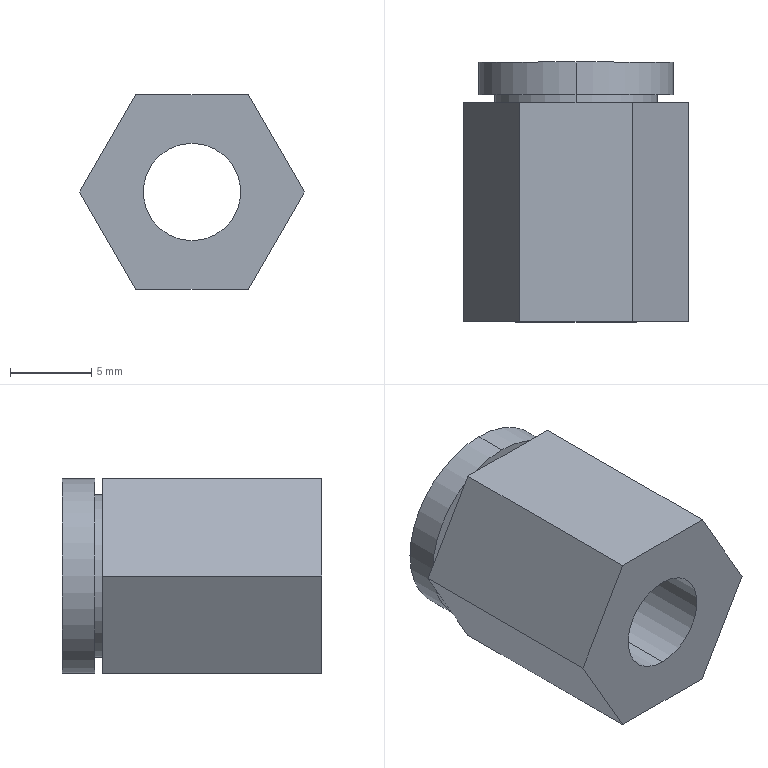Part | SolidWorks | features RefAxis 6, 3DProfileFeature 2, Extrusion 1, HoleWzd 1, Revolution 1 | 1 solid | 16 faces | box 13.856 x 16 x 12 mm | volume 1497 mm3 | plane 10 | cylinder 6 | commonest cylinder face diameters 6 x2 10 x2 12 x2
STEP:
#1=CARTESIAN_POINT('',(0.,16.,3.));
#2=VERTEX_POINT('',#1);
#3=CARTESIAN_POINT('',(0.,16.,-3.));
#4=VERTEX_POINT('',#3);
#5=CARTESIAN_POINT('',(0.,16.,0.));
#6=DIRECTION('',(0.,-1.,0.));
#7=DIRECTION('',(0.,0.,-1.));
#8=AXIS2_PLACEMENT_3D('',#5,#6,#7);
#9=CIRCLE('',#8,3.);
#10=EDGE_CURVE('',#2,#4,#9,.T.);
#11=ORIENTED_EDGE('',*,*,#10,.F.);
#12=CARTESIAN_POINT('',(0.,0.,3.));
#13=VERTEX_POINT('',#12);
#14=CARTESIAN_POINT('',(0.,0.,3.));
#15=DIRECTION('',(0.,-1.,0.));
#16=VECTOR('',#15,1000.);
#17=LINE('',#14,#16);
#18=EDGE_CURVE('',#2,#13,#17,.T.);
#19=ORIENTED_EDGE('',*,*,#18,.T.);
#20=CARTESIAN_POINT('',(0.,0.,-3.));
#21=VERTEX_POINT('',#20);
#22=CARTESIAN_POINT('',(0.,0.,0.));
#23=DIRECTION('',(0.,-1.,0.));
#24=DIRECTION('',(0.,0.,-1.));
#25=AXIS2_PLACEMENT_3D('',#22,#23,#24);
#26=CIRCLE('',#25,3.);
#27=EDGE_CURVE('',#13,#21,#26,.T.);
#28=ORIENTED_EDGE('',*,*,#27,.T.);
#29=CARTESIAN_POINT('',(0.,0.,-3.));
#30=DIRECTION('',(0.,-1.,0.));
#31=VECTOR('',#30,1000.);
#32=LINE('',#29,#31);
#33=EDGE_CURVE('',#4,#21,#32,.T.);
#34=ORIENTED_EDGE('',*,*,#33,.F.);
#35=EDGE_LOOP('',(#11,#19,#28,#34));
#36=FACE_OUTER_BOUND('',#35,.T.);
#37=CARTESIAN_POINT('',(0.,0.,0.));
#38=DIRECTION('',(0.,-1.,0.));
#39=DIRECTION('',(0.,0.,-1.));
#40=AXIS2_PLACEMENT_3D('',#37,#38,#39);
#41=CYLINDRICAL_SURFACE('',#40,3.);
#42=ADVANCED_FACE('',(#36),#41,.F.);
#43=CARTESIAN_POINT('',(0.,13.5,5.));
#44=VERTEX_POINT('',#43);
#45=CARTESIAN_POINT('',(0.,13.5,-5.));
#46=VERTEX_POINT('',#45);
#47=CARTESIAN_POINT('',(0.,13.5,0.));
#48=DIRECTION('',(0.,1.,0.));
#49=DIRECTION('',(0.,0.,1.));
#50=AXIS2_PLACEMENT_3D('',#47,#48,#49);
#51=CIRCLE('',#50,5.);
#52=EDGE_CURVE('',#44,#46,#51,.T.);
#53=ORIENTED_EDGE('',*,*,#52,.T.);
#54=CARTESIAN_POINT('',(0.,14.,-5.));
#55=VERTEX_POINT('',#54);
#56=CARTESIAN_POINT('',(0.,13.5,-5.));
#57=DIRECTION('',(0.,1.,0.));
#58=VECTOR('',#57,1000.);
#59=LINE('',#56,#58);
#60=EDGE_CURVE('',#46,#55,#59,.T.);
#61=ORIENTED_EDGE('',*,*,#60,.T.);
#62=CARTESIAN_POINT('',(0.,14.,5.));
#63=VERTEX_POINT('',#62);
#64=CARTESIAN_POINT('',(0.,14.,0.));
#65=DIRECTION('',(0.,1.,0.));
#66=DIRECTION('',(0.,0.,1.));
#67=AXIS2_PLACEMENT_3D('',#64,#65,#66);
#68=CIRCLE('',#67,5.);
#69=EDGE_CURVE('',#63,#55,#68,.T.);
#70=ORIENTED_EDGE('',*,*,#69,.F.);
#71=CARTESIAN_POINT('',(0.,13.5,5.));
#72=DIRECTION('',(0.,1.,0.));
#73=VECTOR('',#72,1000.);
#74=LINE('',#71,#73);
#75=EDGE_CURVE('',#44,#63,#74,.T.);
#76=ORIENTED_EDGE('',*,*,#75,.F.);
#77=EDGE_LOOP('',(#53,#61,#70,#76));
#78=FACE_OUTER_BOUND('',#77,.T.);
#79=CARTESIAN_POINT('',(0.,13.5,0.));
#80=DIRECTION('',(0.,1.,0.));
#81=DIRECTION('',(0.,0.,1.));
#82=AXIS2_PLACEMENT_3D('',#79,#80,#81);
#83=CYLINDRICAL_SURFACE('',#82,5.);
#84=ADVANCED_FACE('',(#78),#83,.T.);
#85=CARTESIAN_POINT('',(0.,14.,6.));
#86=VERTEX_POINT('',#85);
#87=CARTESIAN_POINT('',(0.,14.,-6.));
#88=VERTEX_POINT('',#87);
#89=CARTESIAN_POINT('',(0.,14.,0.));
#90=DIRECTION('',(0.,1.,0.));
#91=DIRECTION('',(0.,0.,1.));
#92=AXIS2_PLACEMENT_3D('',#89,#90,#91);
#93=CIRCLE('',#92,6.);
#94=EDGE_CURVE('',#86,#88,#93,.T.);
#95=ORIENTED_EDGE('',*,*,#94,.T.);
#96=CARTESIAN_POINT('',(0.,16.,-6.));
#97=VERTEX_POINT('',#96);
#98=CARTESIAN_POINT('',(0.,13.5,-6.));
#99=DIRECTION('',(0.,1.,0.));
#100=VECTOR('',#99,1000.);
#101=LINE('',#98,#100);
#102=EDGE_CURVE('',#88,#97,#101,.T.);
#103=ORIENTED_EDGE('',*,*,#102,.T.);
#104=CARTESIAN_POINT('',(0.,16.,6.));
#105=VERTEX_POINT('',#104);
#106=CARTESIAN_POINT('',(0.,16.,0.));
#107=DIRECTION('',(0.,1.,0.));
#108=DIRECTION('',(0.,0.,1.));
#109=AXIS2_PLACEMENT_3D('',#106,#107,#108);
#110=CIRCLE('',#109,6.);
#111=EDGE_CURVE('',#105,#97,#110,.T.);
#112=ORIENTED_EDGE('',*,*,#111,.F.);
#113=CARTESIAN_POINT('',(0.,13.5,6.));
#114=DIRECTION('',(0.,1.,0.));
#115=VECTOR('',#114,1000.);
#116=LINE('',#113,#115);
#117=EDGE_CURVE('',#86,#105,#116,.T.);
#118=ORIENTED_EDGE('',*,*,#117,.F.);
#119=EDGE_LOOP('',(#95,#103,#112,#118));
#120=FACE_OUTER_BOUND('',#119,.T.);
#121=CARTESIAN_POINT('',(0.,13.5,0.));
#122=DIRECTION('',(0.,1.,0.));
#123=DIRECTION('',(0.,0.,1.));
#124=AXIS2_PLACEMENT_3D('',#121,#122,#123);
#125=CYLINDRICAL_SURFACE('',#124,6.);
#126=ADVANCED_FACE('',(#120),#125,.T.);
#127=CARTESIAN_POINT('',(-3.464,13.5,-6.));
#128=VERTEX_POINT('',#127);
#129=CARTESIAN_POINT('',(-6.928,13.5,0.));
#130=VERTEX_POINT('',#129);
#131=CARTESIAN_POINT('',(-3.464,13.5,-6.));
#132=DIRECTION('',(-0.5,0.,0.866));
#133=VECTOR('',#132,1000.);
#134=LINE('',#131,#133);
#135=EDGE_CURVE('',#128,#130,#134,.T.);
#136=ORIENTED_EDGE('',*,*,#135,.T.);
#137=CARTESIAN_POINT('',(-3.464,13.5,6.));
#138=VERTEX_POINT('',#137);
#139=CARTESIAN_POINT('',(-6.928,13.5,0.));
#140=DIRECTION('',(0.5,0.,0.866));
#141=VECTOR('',#140,1000.);
#142=LINE('',#139,#141);
#143=EDGE_CURVE('',#130,#138,#142,.T.);
#144=ORIENTED_EDGE('',*,*,#143,.T.);
#145=CARTESIAN_POINT('',(3.464,13.5,6.));
#146=VERTEX_POINT('',#145);
#147=CARTESIAN_POINT('',(-3.464,13.5,6.));
#148=DIRECTION('',(1.,0.,0.));
#149=VECTOR('',#148,1000.);
#150=LINE('',#147,#149);
#151=EDGE_CURVE('',#138,#146,#150,.T.);
#152=ORIENTED_EDGE('',*,*,#151,.T.);
#153=CARTESIAN_POINT('',(6.928,13.5,0.));
#154=VERTEX_POINT('',#153);
#155=CARTESIAN_POINT('',(3.464,13.5,6.));
#156=DIRECTION('',(0.5,0.,-0.866));
#157=VECTOR('',#156,1000.);
#158=LINE('',#155,#157);
#159=EDGE_CURVE('',#146,#154,#158,.T.);
#160=ORIENTED_EDGE('',*,*,#159,.T.);
#161=CARTESIAN_POINT('',(3.464,13.5,-6.));
#162=VERTEX_POINT('',#161);
#163=CARTESIAN_POINT('',(6.928,13.5,0.));
#164=DIRECTION('',(-0.5,0.,-0.866));
#165=VECTOR('',#164,1000.);
#166=LINE('',#163,#165);
#167=EDGE_CURVE('',#154,#162,#166,.T.);
#168=ORIENTED_EDGE('',*,*,#167,.T.);
#169=CARTESIAN_POINT('',(3.464,13.5,-6.));
#170=DIRECTION('',(-1.,0.,0.));
#171=VECTOR('',#170,1000.);
#172=LINE('',#169,#171);
#173=EDGE_CURVE('',#162,#128,#172,.T.);
#174=ORIENTED_EDGE('',*,*,#173,.T.);
#175=EDGE_LOOP('',(#136,#144,#152,#160,#168,#174));
#176=FACE_OUTER_BOUND('',#175,.T.);
#177=ORIENTED_EDGE('',*,*,#52,.F.);
#178=CARTESIAN_POINT('',(0.,13.5,0.));
#179=DIRECTION('',(0.,1.,0.));
#180=DIRECTION('',(0.,0.,1.));
#181=AXIS2_PLACEMENT_3D('',#178,#179,#180);
#182=CIRCLE('',#181,5.);
#183=EDGE_CURVE('',#46,#44,#182,.T.);
#184=ORIENTED_EDGE('',*,*,#183,.F.);
#185=EDGE_LOOP('',(#177,#184));
#186=FACE_BOUND('',#185,.T.);
#187=CARTESIAN_POINT('',(0.,13.5,0.));
#188=DIRECTION('',(0.,1.,0.));
#189=DIRECTION('',(0.,0.,1.));
#190=AXIS2_PLACEMENT_3D('',#187,#188,#189);
#191=PLANE('',#190);
#192=ADVANCED_FACE('',(#176,#186),#191,.T.);
#193=CARTESIAN_POINT('',(-3.464,0.,-6.));
#194=VERTEX_POINT('',#193);
#195=CARTESIAN_POINT('',(-6.928,0.,0.));
#196=VERTEX_POINT('',#195);
#197=CARTESIAN_POINT('',(-3.464,0.,-6.));
#198=DIRECTION('',(-0.5,0.,0.866));
#199=VECTOR('',#198,1000.);
#200=LINE('',#197,#199);
#201=EDGE_CURVE('',#194,#196,#200,.T.);
#202=ORIENTED_EDGE('',*,*,#201,.T.);
#203=CARTESIAN_POINT('',(-6.928,13.5,0.));
#204=DIRECTION('',(0.,-1.,0.));
#205=VECTOR('',#204,1000.);
#206=LINE('',#203,#205);
#207=EDGE_CURVE('',#130,#196,#206,.T.);
#208=ORIENTED_EDGE('',*,*,#207,.F.);
#209=ORIENTED_EDGE('',*,*,#135,.F.);
#210=CARTESIAN_POINT('',(-3.464,13.5,-6.));
#211=DIRECTION('',(0.,-1.,0.));
#212=VECTOR('',#211,1000.);
#213=LINE('',#210,#212);
#214=EDGE_CURVE('',#128,#194,#213,.T.);
#215=ORIENTED_EDGE('',*,*,#214,.T.);
#216=EDGE_LOOP('',(#202,#208,#209,#215));
#217=FACE_OUTER_BOUND('',#216,.T.);
#218=CARTESIAN_POINT('',(-3.464,13.5,-6.));
#219=DIRECTION('',(0.866,0.,0.5));
#220=DIRECTION('',(0.5,0.,-0.866));
#221=AXIS2_PLACEMENT_3D('',#218,#219,#220);
#222=PLANE('',#221);
#223=ADVANCED_FACE('',(#217),#222,.F.);
#224=CARTESIAN_POINT('',(-3.464,0.,6.));
#225=VERTEX_POINT('',#224);
#226=CARTESIAN_POINT('',(-6.928,0.,0.));
#227=DIRECTION('',(0.5,0.,0.866));
#228=VECTOR('',#227,1000.);
#229=LINE('',#226,#228);
#230=EDGE_CURVE('',#196,#225,#229,.T.);
#231=ORIENTED_EDGE('',*,*,#230,.T.);
#232=CARTESIAN_POINT('',(-3.464,13.5,6.));
#233=DIRECTION('',(0.,-1.,0.));
#234=VECTOR('',#233,1000.);
#235=LINE('',#232,#234);
#236=EDGE_CURVE('',#138,#225,#235,.T.);
#237=ORIENTED_EDGE('',*,*,#236,.F.);
#238=ORIENTED_EDGE('',*,*,#143,.F.);
#239=ORIENTED_EDGE('',*,*,#207,.T.);
#240=EDGE_LOOP('',(#231,#237,#238,#239));
#241=FACE_OUTER_BOUND('',#240,.T.);
#242=CARTESIAN_POINT('',(-6.928,13.5,0.));
#243=DIRECTION('',(0.866,0.,-0.5));
#244=DIRECTION('',(-0.5,0.,-0.866));
#245=AXIS2_PLACEMENT_3D('',#242,#243,#244);
#246=PLANE('',#245);
#247=ADVANCED_FACE('',(#241),#246,.F.);
#248=CARTESIAN_POINT('',(3.464,0.,6.));
#249=VERTEX_POINT('',#248);
#250=CARTESIAN_POINT('',(-3.464,0.,6.));
#251=DIRECTION('',(1.,0.,0.));
#252=VECTOR('',#251,1000.);
#253=LINE('',#250,#252);
#254=EDGE_CURVE('',#225,#249,#253,.T.);
#255=ORIENTED_EDGE('',*,*,#254,.T.);
#256=CARTESIAN_POINT('',(3.464,13.5,6.));
#257=DIRECTION('',(0.,-1.,0.));
#258=VECTOR('',#257,1000.);
#259=LINE('',#256,#258);
#260=EDGE_CURVE('',#146,#249,#259,.T.);
#261=ORIENTED_EDGE('',*,*,#260,.F.);
#262=ORIENTED_EDGE('',*,*,#151,.F.);
#263=ORIENTED_EDGE('',*,*,#236,.T.);
#264=EDGE_LOOP('',(#255,#261,#262,#263));
#265=FACE_OUTER_BOUND('',#264,.T.);
#266=CARTESIAN_POINT('',(-3.464,13.5,6.));
#267=DIRECTION('',(0.,0.,-1.));
#268=DIRECTION('',(-1.,0.,0.));
#269=AXIS2_PLACEMENT_3D('',#266,#267,#268);
#270=PLANE('',#269);
#271=ADVANCED_FACE('',(#265),#270,.F.);
#272=CARTESIAN_POINT('',(6.928,0.,0.));
#273=VERTEX_POINT('',#272);
#274=CARTESIAN_POINT('',(3.464,0.,6.));
#275=DIRECTION('',(0.5,0.,-0.866));
#276=VECTOR('',#275,1000.);
#277=LINE('',#274,#276);
#278=EDGE_CURVE('',#249,#273,#277,.T.);
#279=ORIENTED_EDGE('',*,*,#278,.T.);
#280=CARTESIAN_POINT('',(6.928,13.5,0.));
#281=DIRECTION('',(0.,-1.,0.));
#282=VECTOR('',#281,1000.);
#283=LINE('',#280,#282);
#284=EDGE_CURVE('',#154,#273,#283,.T.);
#285=ORIENTED_EDGE('',*,*,#284,.F.);
#286=ORIENTED_EDGE('',*,*,#159,.F.);
#287=ORIENTED_EDGE('',*,*,#260,.T.);
#288=EDGE_LOOP('',(#279,#285,#286,#287));
#289=FACE_OUTER_BOUND('',#288,.T.);
#290=CARTESIAN_POINT('',(3.464,13.5,6.));
#291=DIRECTION('',(-0.866,0.,-0.5));
#292=DIRECTION('',(-0.5,0.,0.866));
#293=AXIS2_PLACEMENT_3D('',#290,#291,#292);
#294=PLANE('',#293);
#295=ADVANCED_FACE('',(#289),#294,.F.);
#296=CARTESIAN_POINT('',(3.464,0.,-6.));
#297=VERTEX_POINT('',#296);
#298=CARTESIAN_POINT('',(6.928,0.,0.));
#299=DIRECTION('',(-0.5,0.,-0.866));
#300=VECTOR('',#299,1000.);
#301=LINE('',#298,#300);
#302=EDGE_CURVE('',#273,#297,#301,.T.);
#303=ORIENTED_EDGE('',*,*,#302,.T.);
#304=CARTESIAN_POINT('',(3.464,13.5,-6.));
#305=DIRECTION('',(0.,-1.,0.));
#306=VECTOR('',#305,1000.);
#307=LINE('',#304,#306);
#308=EDGE_CURVE('',#162,#297,#307,.T.);
#309=ORIENTED_EDGE('',*,*,#308,.F.);
#310=ORIENTED_EDGE('',*,*,#167,.F.);
#311=ORIENTED_EDGE('',*,*,#284,.T.);
#312=EDGE_LOOP('',(#303,#309,#310,#311));
#313=FACE_OUTER_BOUND('',#312,.T.);
#314=CARTESIAN_POINT('',(6.928,13.5,0.));
#315=DIRECTION('',(-0.866,0.,0.5));
#316=DIRECTION('',(0.5,0.,0.866));
#317=AXIS2_PLACEMENT_3D('',#314,#315,#316);
#318=PLANE('',#317);
#319=ADVANCED_FACE('',(#313),#318,.F.);
#320=CARTESIAN_POINT('',(3.464,0.,-6.));
#321=DIRECTION('',(-1.,0.,0.));
#322=VECTOR('',#321,1000.);
#323=LINE('',#320,#322);
#324=EDGE_CURVE('',#297,#194,#323,.T.);
#325=ORIENTED_EDGE('',*,*,#324,.T.);
#326=ORIENTED_EDGE('',*,*,#214,.F.);
#327=ORIENTED_EDGE('',*,*,#173,.F.);
#328=ORIENTED_EDGE('',*,*,#308,.T.);
#329=EDGE_LOOP('',(#325,#326,#327,#328));
#330=FACE_OUTER_BOUND('',#329,.T.);
#331=CARTESIAN_POINT('',(3.464,13.5,-6.));
#332=DIRECTION('',(0.,0.,1.));
#333=DIRECTION('',(1.,0.,0.));
#334=AXIS2_PLACEMENT_3D('',#331,#332,#333);
#335=PLANE('',#334);
#336=ADVANCED_FACE('',(#330),#335,.F.);
#337=CARTESIAN_POINT('',(0.,0.,0.));
#338=DIRECTION('',(0.,-1.,0.));
#339=DIRECTION('',(0.,0.,-1.));
#340=AXIS2_PLACEMENT_3D('',#337,#338,#339);
#341=CIRCLE('',#340,3.);
#342=EDGE_CURVE('',#21,#13,#341,.T.);
#343=ORIENTED_EDGE('',*,*,#342,.F.);
#344=ORIENTED_EDGE('',*,*,#27,.F.);
#345=EDGE_LOOP('',(#343,#344));
#346=FACE_BOUND('',#345,.T.);
#347=ORIENTED_EDGE('',*,*,#201,.F.);
#348=ORIENTED_EDGE('',*,*,#324,.F.);
#349=ORIENTED_EDGE('',*,*,#302,.F.);
#350=ORIENTED_EDGE('',*,*,#278,.F.);
#351=ORIENTED_EDGE('',*,*,#254,.F.);
#352=ORIENTED_EDGE('',*,*,#230,.F.);
#353=EDGE_LOOP('',(#347,#348,#349,#350,#351,#352));
#354=FACE_OUTER_BOUND('',#353,.T.);
#355=CARTESIAN_POINT('',(0.,0.,0.));
#356=DIRECTION('',(0.,1.,0.));
#357=DIRECTION('',(0.,0.,1.));
#358=AXIS2_PLACEMENT_3D('',#355,#356,#357);
#359=PLANE('',#358);
#360=ADVANCED_FACE('',(#346,#354),#359,.F.);
#361=CARTESIAN_POINT('',(0.,16.,0.));
#362=DIRECTION('',(0.,-1.,0.));
#363=DIRECTION('',(0.,0.,-1.));
#364=AXIS2_PLACEMENT_3D('',#361,#362,#363);
#365=CIRCLE('',#364,3.);
#366=EDGE_CURVE('',#4,#2,#365,.T.);
#367=ORIENTED_EDGE('',*,*,#366,.T.);
#368=ORIENTED_EDGE('',*,*,#10,.T.);
#369=EDGE_LOOP('',(#367,#368));
#370=FACE_BOUND('',#369,.T.);
#371=ORIENTED_EDGE('',*,*,#111,.T.);
#372=CARTESIAN_POINT('',(0.,16.,0.));
#373=DIRECTION('',(0.,1.,0.));
#374=DIRECTION('',(0.,0.,1.));
#375=AXIS2_PLACEMENT_3D('',#372,#373,#374);
#376=CIRCLE('',#375,6.);
#377=EDGE_CURVE('',#97,#105,#376,.T.);
#378=ORIENTED_EDGE('',*,*,#377,.T.);
#379=EDGE_LOOP('',(#371,#378));
#380=FACE_OUTER_BOUND('',#379,.T.);
#381=CARTESIAN_POINT('',(0.,16.,0.));
#382=DIRECTION('',(0.,-1.,0.));
#383=DIRECTION('',(0.,0.,-1.));
#384=AXIS2_PLACEMENT_3D('',#381,#382,#383);
#385=PLANE('',#384);
#386=ADVANCED_FACE('',(#370,#380),#385,.F.);
#387=ORIENTED_EDGE('',*,*,#102,.F.);
#388=CARTESIAN_POINT('',(0.,14.,0.));
#389=DIRECTION('',(0.,1.,0.));
#390=DIRECTION('',(0.,0.,1.));
#391=AXIS2_PLACEMENT_3D('',#388,#389,#390);
#392=CIRCLE('',#391,6.);
#393=EDGE_CURVE('',#88,#86,#392,.T.);
#394=ORIENTED_EDGE('',*,*,#393,.T.);
#395=ORIENTED_EDGE('',*,*,#117,.T.);
#396=ORIENTED_EDGE('',*,*,#377,.F.);
#397=EDGE_LOOP('',(#387,#394,#395,#396));
#398=FACE_OUTER_BOUND('',#397,.T.);
#399=CARTESIAN_POINT('',(0.,13.5,0.));
#400=DIRECTION('',(0.,1.,0.));
#401=DIRECTION('',(0.,0.,1.));
#402=AXIS2_PLACEMENT_3D('',#399,#400,#401);
#403=CYLINDRICAL_SURFACE('',#402,6.);
#404=ADVANCED_FACE('',(#398),#403,.T.);
#405=ORIENTED_EDGE('',*,*,#94,.F.);
#406=ORIENTED_EDGE('',*,*,#393,.F.);
#407=EDGE_LOOP('',(#405,#406));
#408=FACE_OUTER_BOUND('',#407,.T.);
#409=ORIENTED_EDGE('',*,*,#69,.T.);
#410=CARTESIAN_POINT('',(0.,14.,0.));
#411=DIRECTION('',(0.,1.,0.));
#412=DIRECTION('',(0.,0.,1.));
#413=AXIS2_PLACEMENT_3D('',#410,#411,#412);
#414=CIRCLE('',#413,5.);
#415=EDGE_CURVE('',#55,#63,#414,.T.);
#416=ORIENTED_EDGE('',*,*,#415,.T.);
#417=EDGE_LOOP('',(#409,#416));
#418=FACE_BOUND('',#417,.T.);
#419=CARTESIAN_POINT('',(6.,14.,0.));
#420=DIRECTION('',(0.,1.,0.));
#421=DIRECTION('',(0.,0.,1.));
#422=AXIS2_PLACEMENT_3D('',#419,#420,#421);
#423=PLANE('',#422);
#424=ADVANCED_FACE('',(#408,#418),#423,.F.);
#425=ORIENTED_EDGE('',*,*,#60,.F.);
#426=ORIENTED_EDGE('',*,*,#183,.T.);
#427=ORIENTED_EDGE('',*,*,#75,.T.);
#428=ORIENTED_EDGE('',*,*,#415,.F.);
#429=EDGE_LOOP('',(#425,#426,#427,#428));
#430=FACE_OUTER_BOUND('',#429,.T.);
#431=CARTESIAN_POINT('',(0.,13.5,0.));
#432=DIRECTION('',(0.,1.,0.));
#433=DIRECTION('',(0.,0.,1.));
#434=AXIS2_PLACEMENT_3D('',#431,#432,#433);
#435=CYLINDRICAL_SURFACE('',#434,5.);
#436=ADVANCED_FACE('',(#430),#435,.T.);
#437=ORIENTED_EDGE('',*,*,#18,.F.);
#438=ORIENTED_EDGE('',*,*,#366,.F.);
#439=ORIENTED_EDGE('',*,*,#33,.T.);
#440=ORIENTED_EDGE('',*,*,#342,.T.);
#441=EDGE_LOOP('',(#437,#438,#439,#440));
#442=FACE_OUTER_BOUND('',#441,.T.);
#443=CARTESIAN_POINT('',(0.,0.,0.));
#444=DIRECTION('',(0.,-1.,0.));
#445=DIRECTION('',(0.,0.,-1.));
#446=AXIS2_PLACEMENT_3D('',#443,#444,#445);
#447=CYLINDRICAL_SURFACE('',#446,3.);
#448=ADVANCED_FACE('',(#442),#447,.F.);
#449=CLOSED_SHELL('',(#42,#84,#126,#192,#223,#247,#271,#295,#319,#336,#360,#386,#404,#424,#436,#448));
#450=MANIFOLD_SOLID_BREP('',#449);
#451=CARTESIAN_POINT('',(0.,0.,0.));
#452=DIRECTION('',(0.,0.,1.));
#453=DIRECTION('',(1.,0.,0.));
#454=AXIS2_PLACEMENT_3D('',#451,#452,#453);
#455=(LENGTH_UNIT()NAMED_UNIT(*)SI_UNIT(.MILLI.,.METRE.));
#456=UNCERTAINTY_MEASURE_WITH_UNIT(LENGTH_MEASURE(0.00001),#455,'','');
#457=(NAMED_UNIT(*)PLANE_ANGLE_UNIT()SI_UNIT($,.RADIAN.));
#458=(NAMED_UNIT(*)SI_UNIT($,.STERADIAN.)SOLID_ANGLE_UNIT());
#459=(GEOMETRIC_REPRESENTATION_CONTEXT(3)GLOBAL_UNCERTAINTY_ASSIGNED_CONTEXT((#456))GLOBAL_UNIT_ASSIGNED_CONTEXT((#455,#457,#458))REPRESENTATION_CONTEXT('',''));
#460=ADVANCED_BREP_SHAPE_REPRESENTATION('',(#450,#454),#459);